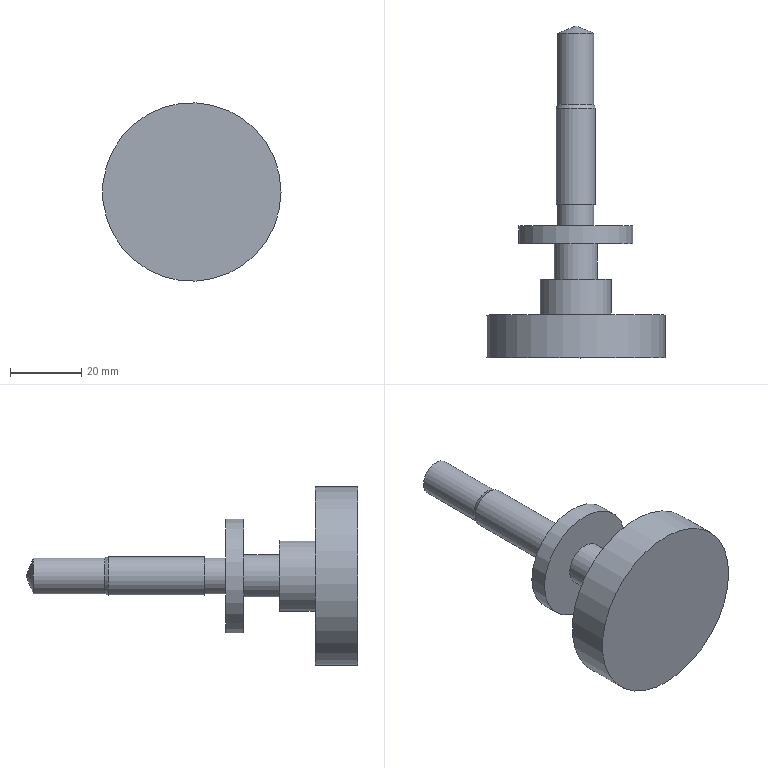Part | NX | features EXTRUDE 7, DATUM_CSYS 5, SKETCH 4, CONE 2, UNITE 1 | 1 solid | 15 faces | box 50 x 93 x 50 mm | volume 36603 mm3 | cylinder 7 | plane 6 | cone 2 | commonest cylinder face diameters 10 x2 11 x1 12 x1 20 x1 32 x1 50 x1
STEP:
#1=CARTESIAN_POINT('',(5.,6.,0.));
#2=VERTEX_POINT('',#1);
#3=CARTESIAN_POINT('',(0.,6.,0.));
#4=DIRECTION('',(0.,1.,0.));
#5=DIRECTION('',(1.,0.,0.));
#6=AXIS2_PLACEMENT_3D('',#3,#4,#5);
#7=CIRCLE('',#6,5.);
#8=EDGE_CURVE('',#2,#2,#7,.T.);
#9=ORIENTED_EDGE('',*,*,#8,.F.);
#10=EDGE_LOOP('',(#9));
#11=FACE_BOUND('',#10,.T.);
#12=CARTESIAN_POINT('',(5.,0.,0.));
#13=VERTEX_POINT('',#12);
#14=CARTESIAN_POINT('',(0.,0.,0.));
#15=DIRECTION('',(0.,1.,0.));
#16=DIRECTION('',(1.,0.,0.));
#17=AXIS2_PLACEMENT_3D('',#14,#15,#16);
#18=CIRCLE('',#17,5.);
#19=EDGE_CURVE('',#13,#13,#18,.T.);
#20=ORIENTED_EDGE('',*,*,#19,.T.);
#21=EDGE_LOOP('',(#20));
#22=FACE_BOUND('',#21,.T.);
#23=CARTESIAN_POINT('',(0.,6.,0.));
#24=DIRECTION('',(0.,-1.,0.));
#25=DIRECTION('',(0.,0.,-1.));
#26=AXIS2_PLACEMENT_3D('',#23,#24,#25);
#27=CYLINDRICAL_SURFACE('',#26,5.);
#28=ADVANCED_FACE('',(#11,#22),#27,.T.);
#29=CARTESIAN_POINT('',(16.,-5.,0.));
#30=VERTEX_POINT('',#29);
#31=CARTESIAN_POINT('',(0.,-5.,0.));
#32=DIRECTION('',(0.,-1.,0.));
#33=DIRECTION('',(1.,0.,0.));
#34=AXIS2_PLACEMENT_3D('',#31,#32,#33);
#35=CIRCLE('',#34,16.);
#36=EDGE_CURVE('',#30,#30,#35,.T.);
#37=ORIENTED_EDGE('',*,*,#36,.F.);
#38=EDGE_LOOP('',(#37));
#39=FACE_BOUND('',#38,.T.);
#40=CARTESIAN_POINT('',(16.,0.,0.));
#41=VERTEX_POINT('',#40);
#42=CARTESIAN_POINT('',(0.,0.,0.));
#43=DIRECTION('',(0.,-1.,0.));
#44=DIRECTION('',(1.,0.,0.));
#45=AXIS2_PLACEMENT_3D('',#42,#43,#44);
#46=CIRCLE('',#45,16.);
#47=EDGE_CURVE('',#41,#41,#46,.T.);
#48=ORIENTED_EDGE('',*,*,#47,.T.);
#49=EDGE_LOOP('',(#48));
#50=FACE_BOUND('',#49,.T.);
#51=CARTESIAN_POINT('',(0.,-5.,0.));
#52=DIRECTION('',(0.,1.,0.));
#53=DIRECTION('',(0.,0.,1.));
#54=AXIS2_PLACEMENT_3D('',#51,#52,#53);
#55=CYLINDRICAL_SURFACE('',#54,16.);
#56=ADVANCED_FACE('',(#39,#50),#55,.T.);
#57=CARTESIAN_POINT('',(6.,-5.,0.));
#58=VERTEX_POINT('',#57);
#59=CARTESIAN_POINT('',(0.,-5.,0.));
#60=DIRECTION('',(0.,1.,0.));
#61=DIRECTION('',(1.,0.,0.));
#62=AXIS2_PLACEMENT_3D('',#59,#60,#61);
#63=CIRCLE('',#62,6.);
#64=EDGE_CURVE('',#58,#58,#63,.T.);
#65=ORIENTED_EDGE('',*,*,#64,.T.);
#66=EDGE_LOOP('',(#65));
#67=FACE_BOUND('',#66,.T.);
#68=ORIENTED_EDGE('',*,*,#36,.T.);
#69=EDGE_LOOP('',(#68));
#70=FACE_BOUND('',#69,.T.);
#71=CARTESIAN_POINT('',(0.,-5.,0.));
#72=DIRECTION('',(0.,-1.,0.));
#73=DIRECTION('',(0.,0.,-1.));
#74=AXIS2_PLACEMENT_3D('',#71,#72,#73);
#75=PLANE('',#74);
#76=ADVANCED_FACE('',(#67,#70),#75,.T.);
#77=ORIENTED_EDGE('',*,*,#19,.F.);
#78=EDGE_LOOP('',(#77));
#79=FACE_BOUND('',#78,.T.);
#80=ORIENTED_EDGE('',*,*,#47,.F.);
#81=EDGE_LOOP('',(#80));
#82=FACE_BOUND('',#81,.T.);
#83=CARTESIAN_POINT('',(0.,0.,0.));
#84=DIRECTION('',(0.,-1.,0.));
#85=DIRECTION('',(0.,0.,-1.));
#86=AXIS2_PLACEMENT_3D('',#83,#84,#85);
#87=PLANE('',#86);
#88=ADVANCED_FACE('',(#79,#82),#87,.F.);
#89=CARTESIAN_POINT('',(6.,-15.,0.));
#90=VERTEX_POINT('',#89);
#91=CARTESIAN_POINT('',(0.,-15.,0.));
#92=DIRECTION('',(0.,1.,0.));
#93=DIRECTION('',(1.,0.,0.));
#94=AXIS2_PLACEMENT_3D('',#91,#92,#93);
#95=CIRCLE('',#94,6.);
#96=EDGE_CURVE('',#90,#90,#95,.T.);
#97=ORIENTED_EDGE('',*,*,#96,.T.);
#98=EDGE_LOOP('',(#97));
#99=FACE_BOUND('',#98,.T.);
#100=ORIENTED_EDGE('',*,*,#64,.F.);
#101=EDGE_LOOP('',(#100));
#102=FACE_BOUND('',#101,.T.);
#103=CARTESIAN_POINT('',(0.,-15.,0.));
#104=DIRECTION('',(0.,1.,0.));
#105=DIRECTION('',(0.,0.,1.));
#106=AXIS2_PLACEMENT_3D('',#103,#104,#105);
#107=CYLINDRICAL_SURFACE('',#106,6.);
#108=ADVANCED_FACE('',(#99,#102),#107,.T.);
#109=CARTESIAN_POINT('',(10.,-25.,0.));
#110=VERTEX_POINT('',#109);
#111=CARTESIAN_POINT('',(0.,-25.,0.));
#112=DIRECTION('',(0.,-1.,0.));
#113=DIRECTION('',(1.,0.,0.));
#114=AXIS2_PLACEMENT_3D('',#111,#112,#113);
#115=CIRCLE('',#114,10.);
#116=EDGE_CURVE('',#110,#110,#115,.T.);
#117=ORIENTED_EDGE('',*,*,#116,.F.);
#118=EDGE_LOOP('',(#117));
#119=FACE_BOUND('',#118,.T.);
#120=CARTESIAN_POINT('',(10.,-15.,0.));
#121=VERTEX_POINT('',#120);
#122=CARTESIAN_POINT('',(0.,-15.,0.));
#123=DIRECTION('',(0.,-1.,0.));
#124=DIRECTION('',(1.,0.,0.));
#125=AXIS2_PLACEMENT_3D('',#122,#123,#124);
#126=CIRCLE('',#125,10.);
#127=EDGE_CURVE('',#121,#121,#126,.T.);
#128=ORIENTED_EDGE('',*,*,#127,.T.);
#129=EDGE_LOOP('',(#128));
#130=FACE_BOUND('',#129,.T.);
#131=CARTESIAN_POINT('',(0.,-25.,0.));
#132=DIRECTION('',(0.,1.,0.));
#133=DIRECTION('',(0.,0.,1.));
#134=AXIS2_PLACEMENT_3D('',#131,#132,#133);
#135=CYLINDRICAL_SURFACE('',#134,10.);
#136=ADVANCED_FACE('',(#119,#130),#135,.T.);
#137=ORIENTED_EDGE('',*,*,#96,.F.);
#138=EDGE_LOOP('',(#137));
#139=FACE_BOUND('',#138,.T.);
#140=ORIENTED_EDGE('',*,*,#127,.F.);
#141=EDGE_LOOP('',(#140));
#142=FACE_BOUND('',#141,.T.);
#143=CARTESIAN_POINT('',(0.,-15.,0.));
#144=DIRECTION('',(0.,-1.,0.));
#145=DIRECTION('',(0.,0.,-1.));
#146=AXIS2_PLACEMENT_3D('',#143,#144,#145);
#147=PLANE('',#146);
#148=ADVANCED_FACE('',(#139,#142),#147,.F.);
#149=CARTESIAN_POINT('',(25.,-37.,0.));
#150=VERTEX_POINT('',#149);
#151=CARTESIAN_POINT('',(0.,-37.,0.));
#152=DIRECTION('',(0.,-1.,0.));
#153=DIRECTION('',(1.,0.,0.));
#154=AXIS2_PLACEMENT_3D('',#151,#152,#153);
#155=CIRCLE('',#154,25.);
#156=EDGE_CURVE('',#150,#150,#155,.T.);
#157=ORIENTED_EDGE('',*,*,#156,.F.);
#158=EDGE_LOOP('',(#157));
#159=FACE_BOUND('',#158,.T.);
#160=CARTESIAN_POINT('',(25.,-25.,0.));
#161=VERTEX_POINT('',#160);
#162=CARTESIAN_POINT('',(0.,-25.,0.));
#163=DIRECTION('',(0.,-1.,0.));
#164=DIRECTION('',(1.,0.,0.));
#165=AXIS2_PLACEMENT_3D('',#162,#163,#164);
#166=CIRCLE('',#165,25.);
#167=EDGE_CURVE('',#161,#161,#166,.T.);
#168=ORIENTED_EDGE('',*,*,#167,.T.);
#169=EDGE_LOOP('',(#168));
#170=FACE_BOUND('',#169,.T.);
#171=CARTESIAN_POINT('',(0.,-37.,0.));
#172=DIRECTION('',(0.,1.,0.));
#173=DIRECTION('',(0.,0.,1.));
#174=AXIS2_PLACEMENT_3D('',#171,#172,#173);
#175=CYLINDRICAL_SURFACE('',#174,25.);
#176=ADVANCED_FACE('',(#159,#170),#175,.T.);
#177=ORIENTED_EDGE('',*,*,#156,.T.);
#178=EDGE_LOOP('',(#177));
#179=FACE_BOUND('',#178,.T.);
#180=CARTESIAN_POINT('',(0.,-37.,0.));
#181=DIRECTION('',(0.,-1.,0.));
#182=DIRECTION('',(0.,0.,-1.));
#183=AXIS2_PLACEMENT_3D('',#180,#181,#182);
#184=PLANE('',#183);
#185=ADVANCED_FACE('',(#179),#184,.T.);
#186=ORIENTED_EDGE('',*,*,#116,.T.);
#187=EDGE_LOOP('',(#186));
#188=FACE_BOUND('',#187,.T.);
#189=ORIENTED_EDGE('',*,*,#167,.F.);
#190=EDGE_LOOP('',(#189));
#191=FACE_BOUND('',#190,.T.);
#192=CARTESIAN_POINT('',(0.,-25.,0.));
#193=DIRECTION('',(0.,-1.,0.));
#194=DIRECTION('',(0.,0.,-1.));
#195=AXIS2_PLACEMENT_3D('',#192,#193,#194);
#196=PLANE('',#195);
#197=ADVANCED_FACE('',(#188,#191),#196,.F.);
#198=CARTESIAN_POINT('',(5.5,33.,0.));
#199=VERTEX_POINT('',#198);
#200=CARTESIAN_POINT('',(0.,33.,0.));
#201=DIRECTION('',(0.,1.,0.));
#202=DIRECTION('',(1.,0.,0.));
#203=AXIS2_PLACEMENT_3D('',#200,#201,#202);
#204=CIRCLE('',#203,5.5);
#205=EDGE_CURVE('',#199,#199,#204,.T.);
#206=ORIENTED_EDGE('',*,*,#205,.F.);
#207=EDGE_LOOP('',(#206));
#208=FACE_BOUND('',#207,.T.);
#209=CARTESIAN_POINT('',(5.5,6.,0.));
#210=VERTEX_POINT('',#209);
#211=CARTESIAN_POINT('',(0.,6.,0.));
#212=DIRECTION('',(0.,1.,0.));
#213=DIRECTION('',(1.,0.,0.));
#214=AXIS2_PLACEMENT_3D('',#211,#212,#213);
#215=CIRCLE('',#214,5.5);
#216=EDGE_CURVE('',#210,#210,#215,.T.);
#217=ORIENTED_EDGE('',*,*,#216,.T.);
#218=EDGE_LOOP('',(#217));
#219=FACE_BOUND('',#218,.T.);
#220=CARTESIAN_POINT('',(0.,33.,0.));
#221=DIRECTION('',(0.,-1.,0.));
#222=DIRECTION('',(0.,0.,-1.));
#223=AXIS2_PLACEMENT_3D('',#220,#221,#222);
#224=CYLINDRICAL_SURFACE('',#223,5.5);
#225=ADVANCED_FACE('',(#208,#219),#224,.T.);
#226=ORIENTED_EDGE('',*,*,#8,.T.);
#227=EDGE_LOOP('',(#226));
#228=FACE_BOUND('',#227,.T.);
#229=ORIENTED_EDGE('',*,*,#216,.F.);
#230=EDGE_LOOP('',(#229));
#231=FACE_BOUND('',#230,.T.);
#232=CARTESIAN_POINT('',(0.,6.,0.));
#233=DIRECTION('',(0.,1.,0.));
#234=DIRECTION('',(0.,0.,1.));
#235=AXIS2_PLACEMENT_3D('',#232,#233,#234);
#236=PLANE('',#235);
#237=ADVANCED_FACE('',(#228,#231),#236,.F.);
#238=CARTESIAN_POINT('',(5.,34.,0.));
#239=VERTEX_POINT('',#238);
#240=CARTESIAN_POINT('',(0.,34.,0.));
#241=DIRECTION('',(0.,1.,0.));
#242=DIRECTION('',(1.,0.,0.));
#243=AXIS2_PLACEMENT_3D('',#240,#241,#242);
#244=CIRCLE('',#243,5.);
#245=EDGE_CURVE('',#239,#239,#244,.T.);
#246=ORIENTED_EDGE('',*,*,#245,.F.);
#247=EDGE_LOOP('',(#246));
#248=FACE_BOUND('',#247,.T.);
#249=ORIENTED_EDGE('',*,*,#205,.T.);
#250=EDGE_LOOP('',(#249));
#251=FACE_BOUND('',#250,.T.);
#252=CARTESIAN_POINT('',(0.,34.,0.));
#253=DIRECTION('',(0.,-1.,0.));
#254=DIRECTION('',(1.,0.,0.));
#255=AXIS2_PLACEMENT_3D('',#252,#253,#254);
#256=CONICAL_SURFACE('',#255,5.,0.4636);
#257=ADVANCED_FACE('',(#248,#251),#256,.T.);
#258=CARTESIAN_POINT('',(5.,54.,0.));
#259=VERTEX_POINT('',#258);
#260=CARTESIAN_POINT('',(0.,54.,0.));
#261=DIRECTION('',(0.,1.,0.));
#262=DIRECTION('',(1.,0.,0.));
#263=AXIS2_PLACEMENT_3D('',#260,#261,#262);
#264=CIRCLE('',#263,5.);
#265=EDGE_CURVE('',#259,#259,#264,.T.);
#266=ORIENTED_EDGE('',*,*,#265,.F.);
#267=EDGE_LOOP('',(#266));
#268=FACE_BOUND('',#267,.T.);
#269=ORIENTED_EDGE('',*,*,#245,.T.);
#270=EDGE_LOOP('',(#269));
#271=FACE_BOUND('',#270,.T.);
#272=CARTESIAN_POINT('',(0.,54.,0.));
#273=DIRECTION('',(0.,-1.,0.));
#274=DIRECTION('',(0.,0.,-1.));
#275=AXIS2_PLACEMENT_3D('',#272,#273,#274);
#276=CYLINDRICAL_SURFACE('',#275,5.);
#277=ADVANCED_FACE('',(#268,#271),#276,.T.);
#278=ORIENTED_EDGE('',*,*,#265,.T.);
#279=EDGE_LOOP('',(#278));
#280=FACE_BOUND('',#279,.T.);
#281=CARTESIAN_POINT('',(0.,56.,0.));
#282=VERTEX_POINT('',#281);
#283=VERTEX_LOOP('',#282);
#284=FACE_BOUND('',#283,.T.);
#285=CARTESIAN_POINT('',(0.,56.,0.));
#286=DIRECTION('',(0.,-1.,0.));
#287=DIRECTION('',(1.,0.,0.));
#288=AXIS2_PLACEMENT_3D('',#285,#286,#287);
#289=CONICAL_SURFACE('',#288,0.,1.19);
#290=ADVANCED_FACE('',(#280,#284),#289,.T.);
#291=CLOSED_SHELL('',(#28,#56,#76,#88,#108,#136,#148,#176,#185,#197,#225,#237,#257,#277,#290));
#292=MANIFOLD_SOLID_BREP('',#291);
#293=(LENGTH_UNIT()NAMED_UNIT(*)SI_UNIT(.MILLI.,.METRE.));
#294=UNCERTAINTY_MEASURE_WITH_UNIT(LENGTH_MEASURE(0.00001),#293,'','');
#295=(NAMED_UNIT(*)PLANE_ANGLE_UNIT()SI_UNIT($,.RADIAN.));
#296=(NAMED_UNIT(*)SI_UNIT($,.STERADIAN.)SOLID_ANGLE_UNIT());
#297=(GEOMETRIC_REPRESENTATION_CONTEXT(3)GLOBAL_UNCERTAINTY_ASSIGNED_CONTEXT((#294))GLOBAL_UNIT_ASSIGNED_CONTEXT((#293,#295,#296))REPRESENTATION_CONTEXT('',''));
#298=ADVANCED_BREP_SHAPE_REPRESENTATION('',(#292),#297);